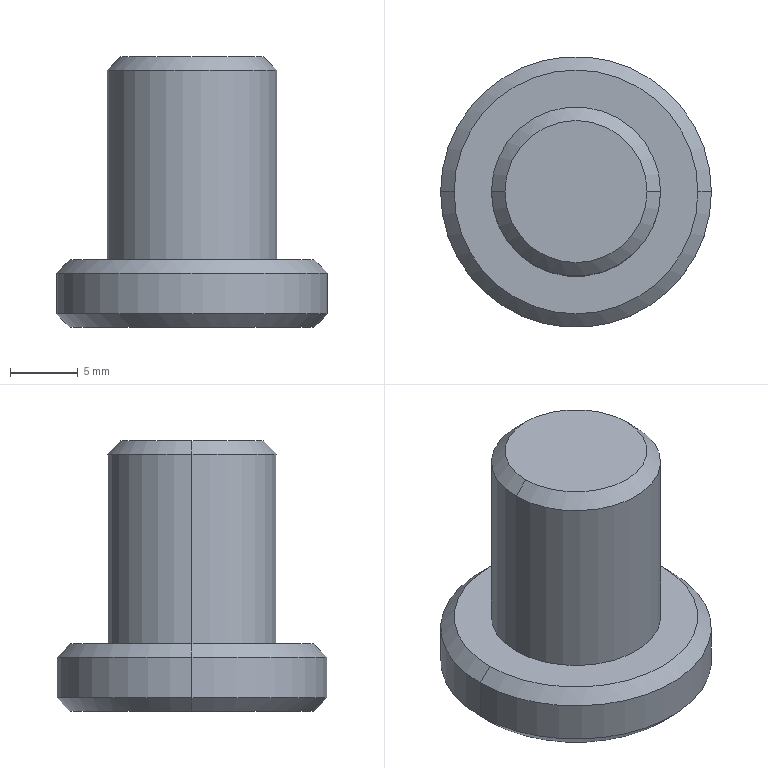Part | SolidWorks | features Chamfer 1, Revolution 1 | 1 solid | 13 faces | box 20 x 20 x 20 mm | volume 3332 mm3 | cone 6 | cylinder 4 | plane 3 | commonest cylinder face diameters 12.5 x2 20 x2
STEP:
#1=CARTESIAN_POINT('',(5.25,0.,0.));
#2=VERTEX_POINT('',#1);
#3=CARTESIAN_POINT('',(-5.25,0.,0.));
#4=VERTEX_POINT('',#3);
#5=CARTESIAN_POINT('',(0.,0.,0.));
#6=DIRECTION('',(0.,0.,1.));
#7=DIRECTION('',(-1.,0.,0.));
#8=AXIS2_PLACEMENT_3D('',#5,#6,#7);
#9=CIRCLE('',#8,5.25);
#10=EDGE_CURVE('',#2,#4,#9,.T.);
#11=ORIENTED_EDGE('',*,*,#10,.F.);
#12=CARTESIAN_POINT('',(6.25,0.,-1.));
#13=VERTEX_POINT('',#12);
#14=CARTESIAN_POINT('',(5.25,0.,0.));
#15=DIRECTION('',(0.7071,0.,-0.7071));
#16=VECTOR('',#15,1000.);
#17=LINE('',#14,#16);
#18=EDGE_CURVE('',#2,#13,#17,.T.);
#19=ORIENTED_EDGE('',*,*,#18,.T.);
#20=CARTESIAN_POINT('',(-6.25,0.,-1.));
#21=VERTEX_POINT('',#20);
#22=CARTESIAN_POINT('',(0.,0.,-1.));
#23=DIRECTION('',(0.,0.,-1.));
#24=DIRECTION('',(-1.,0.,0.));
#25=AXIS2_PLACEMENT_3D('',#22,#23,#24);
#26=CIRCLE('',#25,6.25);
#27=EDGE_CURVE('',#21,#13,#26,.T.);
#28=ORIENTED_EDGE('',*,*,#27,.F.);
#29=CARTESIAN_POINT('',(-5.25,0.,0.));
#30=DIRECTION('',(-0.7071,0.,-0.7071));
#31=VECTOR('',#30,1000.);
#32=LINE('',#29,#31);
#33=EDGE_CURVE('',#4,#21,#32,.T.);
#34=ORIENTED_EDGE('',*,*,#33,.F.);
#35=EDGE_LOOP('',(#11,#19,#28,#34));
#36=FACE_OUTER_BOUND('',#35,.T.);
#37=CARTESIAN_POINT('',(0.,0.,0.));
#38=DIRECTION('',(0.,0.,-1.));
#39=DIRECTION('',(-1.,0.,0.));
#40=AXIS2_PLACEMENT_3D('',#37,#38,#39);
#41=CONICAL_SURFACE('',#40,5.25,0.7854);
#42=ADVANCED_FACE('',(#36),#41,.T.);
#43=CARTESIAN_POINT('',(9.,0.,-15.));
#44=VERTEX_POINT('',#43);
#45=CARTESIAN_POINT('',(-9.,0.,-15.));
#46=VERTEX_POINT('',#45);
#47=CARTESIAN_POINT('',(0.,0.,-15.));
#48=DIRECTION('',(0.,0.,1.));
#49=DIRECTION('',(-1.,0.,0.));
#50=AXIS2_PLACEMENT_3D('',#47,#48,#49);
#51=CIRCLE('',#50,9.);
#52=EDGE_CURVE('',#44,#46,#51,.T.);
#53=ORIENTED_EDGE('',*,*,#52,.F.);
#54=CARTESIAN_POINT('',(10.,0.,-16.));
#55=VERTEX_POINT('',#54);
#56=CARTESIAN_POINT('',(9.,0.,-15.));
#57=DIRECTION('',(0.7071,0.,-0.7071));
#58=VECTOR('',#57,1000.);
#59=LINE('',#56,#58);
#60=EDGE_CURVE('',#44,#55,#59,.T.);
#61=ORIENTED_EDGE('',*,*,#60,.T.);
#62=CARTESIAN_POINT('',(-10.,0.,-16.));
#63=VERTEX_POINT('',#62);
#64=CARTESIAN_POINT('',(0.,0.,-16.));
#65=DIRECTION('',(0.,0.,-1.));
#66=DIRECTION('',(-1.,0.,0.));
#67=AXIS2_PLACEMENT_3D('',#64,#65,#66);
#68=CIRCLE('',#67,10.);
#69=EDGE_CURVE('',#63,#55,#68,.T.);
#70=ORIENTED_EDGE('',*,*,#69,.F.);
#71=CARTESIAN_POINT('',(-9.,0.,-15.));
#72=DIRECTION('',(-0.7071,0.,-0.7071));
#73=VECTOR('',#72,1000.);
#74=LINE('',#71,#73);
#75=EDGE_CURVE('',#46,#63,#74,.T.);
#76=ORIENTED_EDGE('',*,*,#75,.F.);
#77=EDGE_LOOP('',(#53,#61,#70,#76));
#78=FACE_OUTER_BOUND('',#77,.T.);
#79=CARTESIAN_POINT('',(0.,0.,-15.));
#80=DIRECTION('',(0.,0.,-1.));
#81=DIRECTION('',(-1.,0.,0.));
#82=AXIS2_PLACEMENT_3D('',#79,#80,#81);
#83=CONICAL_SURFACE('',#82,9.,0.7854);
#84=ADVANCED_FACE('',(#78),#83,.T.);
#85=CARTESIAN_POINT('',(-9.,0.,-20.));
#86=VERTEX_POINT('',#85);
#87=CARTESIAN_POINT('',(9.,0.,-20.));
#88=VERTEX_POINT('',#87);
#89=CARTESIAN_POINT('',(0.,0.,-20.));
#90=DIRECTION('',(0.,0.,-1.));
#91=DIRECTION('',(1.,0.,0.));
#92=AXIS2_PLACEMENT_3D('',#89,#90,#91);
#93=CIRCLE('',#92,9.);
#94=EDGE_CURVE('',#86,#88,#93,.T.);
#95=ORIENTED_EDGE('',*,*,#94,.F.);
#96=CARTESIAN_POINT('',(-10.,0.,-19.));
#97=VERTEX_POINT('',#96);
#98=CARTESIAN_POINT('',(-10.,0.,-19.));
#99=DIRECTION('',(-0.7071,0.,0.7071));
#100=VECTOR('',#99,1000.);
#101=LINE('',#98,#100);
#102=EDGE_CURVE('',#86,#97,#101,.T.);
#103=ORIENTED_EDGE('',*,*,#102,.T.);
#104=CARTESIAN_POINT('',(10.,0.,-19.));
#105=VERTEX_POINT('',#104);
#106=CARTESIAN_POINT('',(0.,0.,-19.));
#107=DIRECTION('',(0.,0.,1.));
#108=DIRECTION('',(1.,0.,0.));
#109=AXIS2_PLACEMENT_3D('',#106,#107,#108);
#110=CIRCLE('',#109,10.);
#111=EDGE_CURVE('',#105,#97,#110,.T.);
#112=ORIENTED_EDGE('',*,*,#111,.F.);
#113=CARTESIAN_POINT('',(10.,0.,-19.));
#114=DIRECTION('',(0.7071,0.,0.7071));
#115=VECTOR('',#114,1000.);
#116=LINE('',#113,#115);
#117=EDGE_CURVE('',#88,#105,#116,.T.);
#118=ORIENTED_EDGE('',*,*,#117,.F.);
#119=EDGE_LOOP('',(#95,#103,#112,#118));
#120=FACE_OUTER_BOUND('',#119,.T.);
#121=CARTESIAN_POINT('',(0.,0.,-19.));
#122=DIRECTION('',(0.,0.,1.));
#123=DIRECTION('',(1.,0.,0.));
#124=AXIS2_PLACEMENT_3D('',#121,#122,#123);
#125=CONICAL_SURFACE('',#124,10.,0.7854);
#126=ADVANCED_FACE('',(#120),#125,.T.);
#127=CARTESIAN_POINT('',(6.25,0.,-15.));
#128=VERTEX_POINT('',#127);
#129=CARTESIAN_POINT('',(-6.25,0.,-15.));
#130=VERTEX_POINT('',#129);
#131=CARTESIAN_POINT('',(0.,0.,-15.));
#132=DIRECTION('',(0.,0.,1.));
#133=DIRECTION('',(1.,0.,0.));
#134=AXIS2_PLACEMENT_3D('',#131,#132,#133);
#135=CIRCLE('',#134,6.25);
#136=EDGE_CURVE('',#128,#130,#135,.T.);
#137=ORIENTED_EDGE('',*,*,#136,.T.);
#138=CARTESIAN_POINT('',(-6.25,0.,0.));
#139=DIRECTION('',(0.,0.,1.));
#140=VECTOR('',#139,1000.);
#141=LINE('',#138,#140);
#142=EDGE_CURVE('',#130,#21,#141,.T.);
#143=ORIENTED_EDGE('',*,*,#142,.T.);
#144=ORIENTED_EDGE('',*,*,#27,.T.);
#145=CARTESIAN_POINT('',(6.25,0.,0.));
#146=DIRECTION('',(0.,0.,1.));
#147=VECTOR('',#146,1000.);
#148=LINE('',#145,#147);
#149=EDGE_CURVE('',#128,#13,#148,.T.);
#150=ORIENTED_EDGE('',*,*,#149,.F.);
#151=EDGE_LOOP('',(#137,#143,#144,#150));
#152=FACE_OUTER_BOUND('',#151,.T.);
#153=CARTESIAN_POINT('',(0.,0.,0.));
#154=DIRECTION('',(0.,0.,1.));
#155=DIRECTION('',(1.,0.,0.));
#156=AXIS2_PLACEMENT_3D('',#153,#154,#155);
#157=CYLINDRICAL_SURFACE('',#156,6.25);
#158=ADVANCED_FACE('',(#152),#157,.T.);
#159=ORIENTED_EDGE('',*,*,#111,.T.);
#160=CARTESIAN_POINT('',(-10.,0.,0.));
#161=DIRECTION('',(0.,0.,1.));
#162=VECTOR('',#161,1000.);
#163=LINE('',#160,#162);
#164=EDGE_CURVE('',#97,#63,#163,.T.);
#165=ORIENTED_EDGE('',*,*,#164,.T.);
#166=ORIENTED_EDGE('',*,*,#69,.T.);
#167=CARTESIAN_POINT('',(10.,0.,0.));
#168=DIRECTION('',(0.,0.,1.));
#169=VECTOR('',#168,1000.);
#170=LINE('',#167,#169);
#171=EDGE_CURVE('',#105,#55,#170,.T.);
#172=ORIENTED_EDGE('',*,*,#171,.F.);
#173=EDGE_LOOP('',(#159,#165,#166,#172));
#174=FACE_OUTER_BOUND('',#173,.T.);
#175=CARTESIAN_POINT('',(0.,0.,0.));
#176=DIRECTION('',(0.,0.,1.));
#177=DIRECTION('',(1.,0.,0.));
#178=AXIS2_PLACEMENT_3D('',#175,#176,#177);
#179=CYLINDRICAL_SURFACE('',#178,10.);
#180=ADVANCED_FACE('',(#174),#179,.T.);
#181=CARTESIAN_POINT('',(0.,0.,-20.));
#182=DIRECTION('',(0.,0.,-1.));
#183=DIRECTION('',(1.,0.,0.));
#184=AXIS2_PLACEMENT_3D('',#181,#182,#183);
#185=CIRCLE('',#184,9.);
#186=EDGE_CURVE('',#88,#86,#185,.T.);
#187=ORIENTED_EDGE('',*,*,#186,.T.);
#188=ORIENTED_EDGE('',*,*,#94,.T.);
#189=EDGE_LOOP('',(#187,#188));
#190=FACE_OUTER_BOUND('',#189,.T.);
#191=CARTESIAN_POINT('',(0.,0.,-20.));
#192=DIRECTION('',(0.,0.,1.));
#193=DIRECTION('',(1.,0.,0.));
#194=AXIS2_PLACEMENT_3D('',#191,#192,#193);
#195=PLANE('',#194);
#196=ADVANCED_FACE('',(#190),#195,.F.);
#197=ORIENTED_EDGE('',*,*,#164,.F.);
#198=CARTESIAN_POINT('',(0.,0.,-19.));
#199=DIRECTION('',(0.,0.,1.));
#200=DIRECTION('',(1.,0.,0.));
#201=AXIS2_PLACEMENT_3D('',#198,#199,#200);
#202=CIRCLE('',#201,10.);
#203=EDGE_CURVE('',#97,#105,#202,.T.);
#204=ORIENTED_EDGE('',*,*,#203,.T.);
#205=ORIENTED_EDGE('',*,*,#171,.T.);
#206=CARTESIAN_POINT('',(0.,0.,-16.));
#207=DIRECTION('',(0.,0.,-1.));
#208=DIRECTION('',(-1.,0.,0.));
#209=AXIS2_PLACEMENT_3D('',#206,#207,#208);
#210=CIRCLE('',#209,10.);
#211=EDGE_CURVE('',#55,#63,#210,.T.);
#212=ORIENTED_EDGE('',*,*,#211,.T.);
#213=EDGE_LOOP('',(#197,#204,#205,#212));
#214=FACE_OUTER_BOUND('',#213,.T.);
#215=CARTESIAN_POINT('',(0.,0.,0.));
#216=DIRECTION('',(0.,0.,1.));
#217=DIRECTION('',(1.,0.,0.));
#218=AXIS2_PLACEMENT_3D('',#215,#216,#217);
#219=CYLINDRICAL_SURFACE('',#218,10.);
#220=ADVANCED_FACE('',(#214),#219,.T.);
#221=CARTESIAN_POINT('',(0.,0.,-15.));
#222=DIRECTION('',(0.,0.,1.));
#223=DIRECTION('',(-1.,0.,0.));
#224=AXIS2_PLACEMENT_3D('',#221,#222,#223);
#225=CIRCLE('',#224,9.);
#226=EDGE_CURVE('',#46,#44,#225,.T.);
#227=ORIENTED_EDGE('',*,*,#226,.T.);
#228=ORIENTED_EDGE('',*,*,#52,.T.);
#229=EDGE_LOOP('',(#227,#228));
#230=FACE_OUTER_BOUND('',#229,.T.);
#231=ORIENTED_EDGE('',*,*,#136,.F.);
#232=CARTESIAN_POINT('',(0.,0.,-15.));
#233=DIRECTION('',(0.,0.,1.));
#234=DIRECTION('',(1.,0.,0.));
#235=AXIS2_PLACEMENT_3D('',#232,#233,#234);
#236=CIRCLE('',#235,6.25);
#237=EDGE_CURVE('',#130,#128,#236,.T.);
#238=ORIENTED_EDGE('',*,*,#237,.F.);
#239=EDGE_LOOP('',(#231,#238));
#240=FACE_BOUND('',#239,.T.);
#241=CARTESIAN_POINT('',(0.,10.,-15.));
#242=DIRECTION('',(0.,0.,-1.));
#243=DIRECTION('',(-1.,0.,0.));
#244=AXIS2_PLACEMENT_3D('',#241,#242,#243);
#245=PLANE('',#244);
#246=ADVANCED_FACE('',(#230,#240),#245,.F.);
#247=ORIENTED_EDGE('',*,*,#142,.F.);
#248=ORIENTED_EDGE('',*,*,#237,.T.);
#249=ORIENTED_EDGE('',*,*,#149,.T.);
#250=CARTESIAN_POINT('',(0.,0.,-1.));
#251=DIRECTION('',(0.,0.,-1.));
#252=DIRECTION('',(-1.,0.,0.));
#253=AXIS2_PLACEMENT_3D('',#250,#251,#252);
#254=CIRCLE('',#253,6.25);
#255=EDGE_CURVE('',#13,#21,#254,.T.);
#256=ORIENTED_EDGE('',*,*,#255,.T.);
#257=EDGE_LOOP('',(#247,#248,#249,#256));
#258=FACE_OUTER_BOUND('',#257,.T.);
#259=CARTESIAN_POINT('',(0.,0.,0.));
#260=DIRECTION('',(0.,0.,1.));
#261=DIRECTION('',(1.,0.,0.));
#262=AXIS2_PLACEMENT_3D('',#259,#260,#261);
#263=CYLINDRICAL_SURFACE('',#262,6.25);
#264=ADVANCED_FACE('',(#258),#263,.T.);
#265=CARTESIAN_POINT('',(0.,0.,0.));
#266=DIRECTION('',(0.,0.,1.));
#267=DIRECTION('',(-1.,0.,0.));
#268=AXIS2_PLACEMENT_3D('',#265,#266,#267);
#269=CIRCLE('',#268,5.25);
#270=EDGE_CURVE('',#4,#2,#269,.T.);
#271=ORIENTED_EDGE('',*,*,#270,.T.);
#272=ORIENTED_EDGE('',*,*,#10,.T.);
#273=EDGE_LOOP('',(#271,#272));
#274=FACE_OUTER_BOUND('',#273,.T.);
#275=CARTESIAN_POINT('',(0.,6.25,0.));
#276=DIRECTION('',(0.,0.,-1.));
#277=DIRECTION('',(-1.,0.,0.));
#278=AXIS2_PLACEMENT_3D('',#275,#276,#277);
#279=PLANE('',#278);
#280=ADVANCED_FACE('',(#274),#279,.F.);
#281=ORIENTED_EDGE('',*,*,#102,.F.);
#282=ORIENTED_EDGE('',*,*,#186,.F.);
#283=ORIENTED_EDGE('',*,*,#117,.T.);
#284=ORIENTED_EDGE('',*,*,#203,.F.);
#285=EDGE_LOOP('',(#281,#282,#283,#284));
#286=FACE_OUTER_BOUND('',#285,.T.);
#287=CARTESIAN_POINT('',(0.,0.,-19.));
#288=DIRECTION('',(0.,0.,1.));
#289=DIRECTION('',(1.,0.,0.));
#290=AXIS2_PLACEMENT_3D('',#287,#288,#289);
#291=CONICAL_SURFACE('',#290,10.,0.7854);
#292=ADVANCED_FACE('',(#286),#291,.T.);
#293=ORIENTED_EDGE('',*,*,#60,.F.);
#294=ORIENTED_EDGE('',*,*,#226,.F.);
#295=ORIENTED_EDGE('',*,*,#75,.T.);
#296=ORIENTED_EDGE('',*,*,#211,.F.);
#297=EDGE_LOOP('',(#293,#294,#295,#296));
#298=FACE_OUTER_BOUND('',#297,.T.);
#299=CARTESIAN_POINT('',(0.,0.,-15.));
#300=DIRECTION('',(0.,0.,-1.));
#301=DIRECTION('',(-1.,0.,0.));
#302=AXIS2_PLACEMENT_3D('',#299,#300,#301);
#303=CONICAL_SURFACE('',#302,9.,0.7854);
#304=ADVANCED_FACE('',(#298),#303,.T.);
#305=ORIENTED_EDGE('',*,*,#18,.F.);
#306=ORIENTED_EDGE('',*,*,#270,.F.);
#307=ORIENTED_EDGE('',*,*,#33,.T.);
#308=ORIENTED_EDGE('',*,*,#255,.F.);
#309=EDGE_LOOP('',(#305,#306,#307,#308));
#310=FACE_OUTER_BOUND('',#309,.T.);
#311=CARTESIAN_POINT('',(0.,0.,0.));
#312=DIRECTION('',(0.,0.,-1.));
#313=DIRECTION('',(-1.,0.,0.));
#314=AXIS2_PLACEMENT_3D('',#311,#312,#313);
#315=CONICAL_SURFACE('',#314,5.25,0.7854);
#316=ADVANCED_FACE('',(#310),#315,.T.);
#317=CLOSED_SHELL('',(#42,#84,#126,#158,#180,#196,#220,#246,#264,#280,#292,#304,#316));
#318=MANIFOLD_SOLID_BREP('',#317);
#319=CARTESIAN_POINT('',(0.,0.,0.));
#320=DIRECTION('',(0.,0.,1.));
#321=DIRECTION('',(1.,0.,0.));
#322=AXIS2_PLACEMENT_3D('',#319,#320,#321);
#323=(LENGTH_UNIT()NAMED_UNIT(*)SI_UNIT(.MILLI.,.METRE.));
#324=UNCERTAINTY_MEASURE_WITH_UNIT(LENGTH_MEASURE(0.00001),#323,'','');
#325=(NAMED_UNIT(*)PLANE_ANGLE_UNIT()SI_UNIT($,.RADIAN.));
#326=(NAMED_UNIT(*)SI_UNIT($,.STERADIAN.)SOLID_ANGLE_UNIT());
#327=(GEOMETRIC_REPRESENTATION_CONTEXT(3)GLOBAL_UNCERTAINTY_ASSIGNED_CONTEXT((#324))GLOBAL_UNIT_ASSIGNED_CONTEXT((#323,#325,#326))REPRESENTATION_CONTEXT('',''));
#328=ADVANCED_BREP_SHAPE_REPRESENTATION('',(#318,#322),#327);